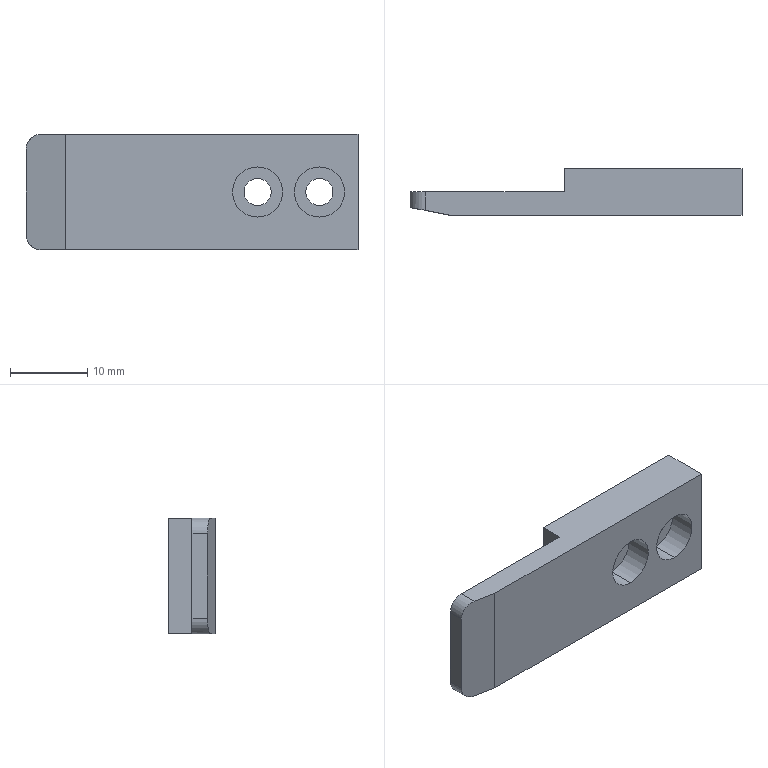Part | STEP file | 0246_206_Lever | 1 solid | 21 faces | box 43 x 6 x 15 mm | volume 2647 mm3 | plane 11 | cylinder 10 | commonest cylinder face diameters 3.5 x4 6.5 x4 4 x2